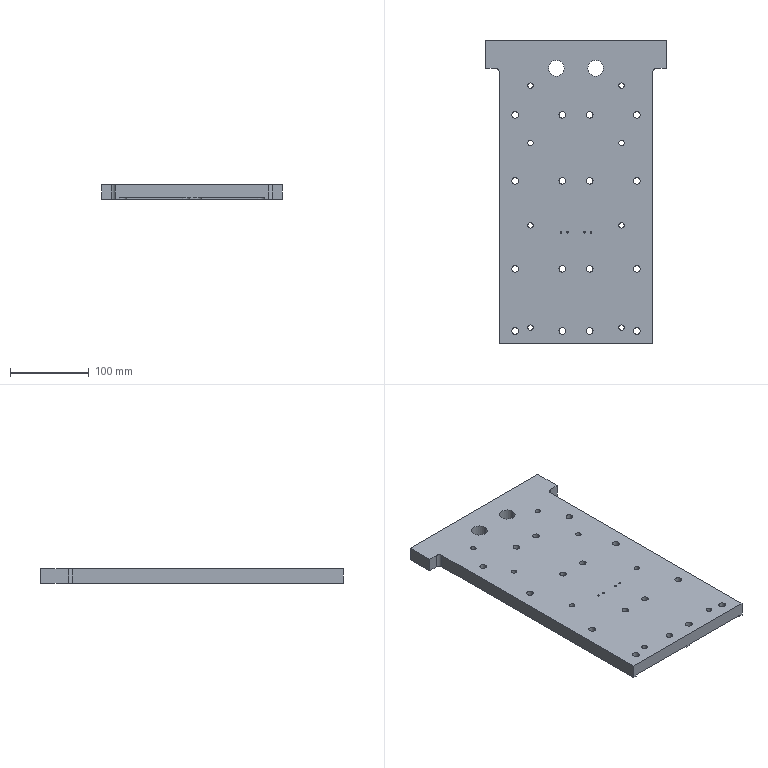NC program | NX | posted with a generic post | part box 230 x 385 x 18 mm
Lines 84 to 1017 of 3056:
(ZLEVEL_PROFILE , TOOL : D10)
N154 T15 M6
N156 G54
N158 G17 G0 G90 X-67.117 Y102.6 S9500 M3
N160 G43 Z30. H15
N162 Z1.5
N164 G94 G1 X-20.05 Z-0.967 F1000.
N166 X152.4 F3000.
N168 Y115.
N170 G2 X157.5 Y120.1 R5.1
N172 G1 X192.5
N174 G2 X197.6 Y115. R5.1
N176 G1 Y-115.
N178 G2 X192.5 Y-120.1 R5.1
N180 G1 X157.5
N182 G2 X152.4 Y-115. R5.1
N184 G1 Y-102.6
N186 X-192.5
N188 G2 X-197.6 Y-97.5 R5.1
N190 G1 Y97.5
N192 G2 X-192.5 Y102.6 R5.1
N194 G1 X-20.05
N196 X152.4 Z-1.099
N198 Y115. Z-1.109
N200 X152.425 Y115.5
N202 X152.498 Y115.995 Z-1.11
N204 X152.62 Y116.48
N206 X152.788 Y116.952
N208 X153.002 Y117.404 Z-1.111
N210 X153.26 Y117.833
N212 X153.558 Y118.235
N214 X153.894 Y118.606 Z-1.112
N216 X154.265 Y118.942
N218 X154.667 Y119.24 Z-1.113
N220 X155.096 Y119.498
N222 X155.548 Y119.712
N224 X156.02 Y119.88 Z-1.114
N226 X156.505 Y120.002
N228 X157. Y120.075 Z-1.115
N230 X157.5 Y120.1
N232 X192.5 Z-1.142
N234 X193. Y120.075
N236 X193.495 Y120.002 Z-1.143
N238 X193.98 Y119.88
N240 X194.452 Y119.712
N242 X194.904 Y119.498 Z-1.144
N244 X195.333 Y119.24
N246 X195.735 Y118.942
N248 X196.106 Y118.606 Z-1.145
N250 X196.442 Y118.235
N252 X196.74 Y117.833 Z-1.146
N254 X196.998 Y117.404
N256 X197.212 Y116.952
N258 X197.38 Y116.48 Z-1.147
N260 X197.502 Y115.995
N262 X197.575 Y115.5 Z-1.148
N264 X197.6 Y115.
N266 Y-115. Z-1.325
N268 X197.575 Y-115.5
N270 X197.502 Y-115.995 Z-1.326
N272 X197.38 Y-116.48
N274 X197.212 Y-116.952
N276 X196.998 Y-117.404 Z-1.327
N278 X196.74 Y-117.833
N280 X196.442 Y-118.235
N282 X196.106 Y-118.606 Z-1.328
N284 X195.735 Y-118.942
N286 X195.333 Y-119.24 Z-1.329
N288 X194.904 Y-119.498
N290 X194.452 Y-119.712
N292 X193.98 Y-119.88 Z-1.33
N294 X193.495 Y-120.002
N296 X193. Y-120.075 Z-1.331
N298 X192.5 Y-120.1
N300 X157.5 Z-1.358
N302 X157. Y-120.075
N304 X156.505 Y-120.002 Z-1.359
N306 X156.02 Y-119.88
N308 X155.548 Y-119.712
N310 X155.096 Y-119.498 Z-1.36
N312 X154.667 Y-119.24
N314 X154.265 Y-118.942
N316 X153.894 Y-118.606 Z-1.361
N318 X153.558 Y-118.235
N320 X153.26 Y-117.833 Z-1.362
N322 X153.002 Y-117.404
N324 X152.788 Y-116.952
N326 X152.62 Y-116.48 Z-1.363
N328 X152.498 Y-115.995
N330 X152.425 Y-115.5 Z-1.364
N332 X152.4 Y-115.
N334 Y-102.6 Z-1.373
N336 X-192.5 Z-1.639
N338 X-193. Y-102.575
N340 X-193.495 Y-102.502
N342 X-193.98 Y-102.38 Z-1.64
N344 X-194.452 Y-102.212
N346 X-194.904 Y-101.998 Z-1.641
N348 X-195.333 Y-101.74
N350 X-195.735 Y-101.442
N352 X-196.106 Y-101.106 Z-1.642
N354 X-196.442 Y-100.735
N356 X-196.74 Y-100.333
N358 X-196.998 Y-99.904 Z-1.643
N360 X-197.212 Y-99.452
N362 X-197.38 Y-98.98 Z-1.644
N364 X-197.502 Y-98.495
N366 X-197.575 Y-98.
N368 X-197.6 Y-97.5 Z-1.645
N370 Y97.5 Z-1.795
N372 X-197.575 Y98.
N374 X-197.502 Y98.495
N376 X-197.38 Y98.98 Z-1.796
N378 X-197.212 Y99.452
N380 X-196.998 Y99.904 Z-1.797
N382 X-196.74 Y100.333
N384 X-196.442 Y100.735
N386 X-196.106 Y101.106 Z-1.798
N388 X-195.735 Y101.442
N390 X-195.333 Y101.74
N392 X-194.904 Y101.998 Z-1.799
N394 X-194.452 Y102.212
N396 X-193.98 Y102.38 Z-1.8
N398 X-193.495 Y102.502
N400 X-193. Y102.575
N402 X-192.5 Y102.6 Z-1.801
N404 X-20.05 Z-1.933
N406 X152.4 Z-2.066
N408 Y115. Z-2.075
N410 X152.425 Y115.5 Z-2.076
N412 X152.498 Y115.995
N414 X152.62 Y116.48 Z-2.077
N416 X152.788 Y116.952
N418 X153.002 Y117.404
N420 X153.26 Y117.833 Z-2.078
N422 X153.558 Y118.235
N424 X153.894 Y118.606
N426 X154.265 Y118.942 Z-2.079
N428 X154.667 Y119.24
N430 X155.096 Y119.498 Z-2.08
N432 X155.548 Y119.712
N434 X156.02 Y119.88
N436 X156.505 Y120.002 Z-2.081
N438 X157. Y120.075
N440 X157.5 Y120.1 Z-2.082
N442 X192.5 Z-2.108
N444 X193. Y120.075 Z-2.109
N446 X193.495 Y120.002
N448 X193.98 Y119.88 Z-2.11
N450 X194.452 Y119.712
N452 X194.904 Y119.498
N454 X195.333 Y119.24 Z-2.111
N456 X195.735 Y118.942
N458 X196.106 Y118.606 Z-2.112
N460 X196.442 Y118.235
N462 X196.74 Y117.833
N464 X196.998 Y117.404 Z-2.113
N466 X197.212 Y116.952
N468 X197.38 Y116.48
N470 X197.502 Y115.995 Z-2.114
N472 X197.575 Y115.5
N474 X197.6 Y115. Z-2.115
N476 Y-115. Z-2.291
N478 X197.575 Y-115.5 Z-2.292
N480 X197.502 Y-115.995
N482 X197.38 Y-116.48 Z-2.293
N484 X197.212 Y-116.952
N486 X196.998 Y-117.404
N488 X196.74 Y-117.833 Z-2.294
N490 X196.442 Y-118.235
N492 X196.106 Y-118.606
N494 X195.735 Y-118.942 Z-2.295
N496 X195.333 Y-119.24
N498 X194.904 Y-119.498 Z-2.296
N500 X194.452 Y-119.712
N502 X193.98 Y-119.88
N504 X193.495 Y-120.002 Z-2.297
N506 X193. Y-120.075
N508 X192.5 Y-120.1 Z-2.298
N510 X157.5 Z-2.324
N512 X157. Y-120.075 Z-2.325
N514 X156.505 Y-120.002
N516 X156.02 Y-119.88 Z-2.326
N518 X155.548 Y-119.712
N520 X155.096 Y-119.498
N522 X154.667 Y-119.24 Z-2.327
N524 X154.265 Y-118.942
N526 X153.894 Y-118.606 Z-2.328
N528 X153.558 Y-118.235
N530 X153.26 Y-117.833
N532 X153.002 Y-117.404 Z-2.329
N534 X152.788 Y-116.952
N536 X152.62 Y-116.48
N538 X152.498 Y-115.995 Z-2.33
N540 X152.425 Y-115.5
N542 X152.4 Y-115. Z-2.331
N544 Y-102.6 Z-2.34
N546 X-192.5 Z-2.605
N548 X-193. Y-102.575 Z-2.606
N550 X-193.495 Y-102.502
N552 X-193.98 Y-102.38
N554 X-194.452 Y-102.212 Z-2.607
N556 X-194.904 Y-101.998
N558 X-195.333 Y-101.74 Z-2.608
N560 X-195.735 Y-101.442
N562 X-196.106 Y-101.106
N564 X-196.442 Y-100.735 Z-2.609
N566 X-196.74 Y-100.333
N568 X-196.998 Y-99.904
N570 X-197.212 Y-99.452 Z-2.61
N572 X-197.38 Y-98.98
N574 X-197.502 Y-98.495 Z-2.611
N576 X-197.575 Y-98.
N578 X-197.6 Y-97.5
N580 Y97.5 Z-2.761
N582 X-197.575 Y98. Z-2.762
N584 X-197.502 Y98.495
N586 X-197.38 Y98.98
N588 X-197.212 Y99.452 Z-2.763
N590 X-196.998 Y99.904
N592 X-196.74 Y100.333 Z-2.764
N594 X-196.442 Y100.735
N596 X-196.106 Y101.106
N598 X-195.735 Y101.442 Z-2.765
N600 X-195.333 Y101.74
N602 X-194.904 Y101.998 Z-2.766
N604 X-194.452 Y102.212
N606 X-193.98 Y102.38
N608 X-193.495 Y102.502 Z-2.767
N610 X-193. Y102.575
N612 X-192.5 Y102.6
N614 X-20.05 Z-2.9
N616 X152.4 Z-3.033
N618 Y115. Z-3.042
N620 X152.425 Y115.5
N622 X152.498 Y115.995 Z-3.043
N624 X152.62 Y116.48
N626 X152.788 Y116.952 Z-3.044
N628 X153.002 Y117.404
N630 X153.26 Y117.833
N632 X153.558 Y118.235 Z-3.045
N634 X153.894 Y118.606
N636 X154.265 Y118.942 Z-3.046
N638 X154.667 Y119.24
N640 X155.096 Y119.498
N642 X155.548 Y119.712 Z-3.047
N644 X156.02 Y119.88
N646 X156.505 Y120.002
N648 X157. Y120.075 Z-3.048
N650 X157.5 Y120.1
N652 X192.5 Z-3.075
N654 X193. Y120.075 Z-3.076
N656 X193.495 Y120.002
N658 X193.98 Y119.88
N660 X194.452 Y119.712 Z-3.077
N662 X194.904 Y119.498
N664 X195.333 Y119.24
N666 X195.735 Y118.942 Z-3.078
N668 X196.106 Y118.606
N670 X196.442 Y118.235 Z-3.079
N672 X196.74 Y117.833
N674 X196.998 Y117.404
N676 X197.212 Y116.952 Z-3.08
N678 X197.38 Y116.48
N680 X197.502 Y115.995 Z-3.081
N682 X197.575 Y115.5
N684 X197.6 Y115.
N686 Y-115. Z-3.258
N688 X197.575 Y-115.5
N690 X197.502 Y-115.995 Z-3.259
N692 X197.38 Y-116.48
N694 X197.212 Y-116.952 Z-3.26
N696 X196.998 Y-117.404
N698 X196.74 Y-117.833
N700 X196.442 Y-118.235 Z-3.261
N702 X196.106 Y-118.606
N704 X195.735 Y-118.942 Z-3.262
N706 X195.333 Y-119.24
N708 X194.904 Y-119.498
N710 X194.452 Y-119.712 Z-3.263
N712 X193.98 Y-119.88
N714 X193.495 Y-120.002
N716 X193. Y-120.075 Z-3.264
N718 X192.5 Y-120.1
N720 X157.5 Z-3.291
N722 X157. Y-120.075 Z-3.292
N724 X156.505 Y-120.002
N726 X156.02 Y-119.88
N728 X155.548 Y-119.712 Z-3.293
N730 X155.096 Y-119.498
N732 X154.667 Y-119.24
N734 X154.265 Y-118.942 Z-3.294
N736 X153.894 Y-118.606
N738 X153.558 Y-118.235 Z-3.295
N740 X153.26 Y-117.833
N742 X153.002 Y-117.404
N744 X152.788 Y-116.952 Z-3.296
N746 X152.62 Y-116.48
N748 X152.498 Y-115.995 Z-3.297
N750 X152.425 Y-115.5
N752 X152.4 Y-115.
N754 Y-102.6 Z-3.307
N756 X-192.5 Z-3.572
N758 X-193. Y-102.575
N760 X-193.495 Y-102.502 Z-3.573
N762 X-193.98 Y-102.38
N764 X-194.452 Y-102.212
N766 X-194.904 Y-101.998 Z-3.574
N768 X-195.333 Y-101.74
N770 X-195.735 Y-101.442 Z-3.575
N772 X-196.106 Y-101.106
N774 X-196.442 Y-100.735
N776 X-196.74 Y-100.333 Z-3.576
N778 X-196.998 Y-99.904
N780 X-197.212 Y-99.452 Z-3.577
N782 X-197.38 Y-98.98
N784 X-197.502 Y-98.495
N786 X-197.575 Y-98. Z-3.578
N788 X-197.6 Y-97.5
N790 Y97.5 Z-3.728
N792 X-197.575 Y98.
N794 X-197.502 Y98.495 Z-3.729
N796 X-197.38 Y98.98
N798 X-197.212 Y99.452 Z-3.73
N800 X-196.998 Y99.904
N802 X-196.74 Y100.333
N804 X-196.442 Y100.735 Z-3.731
N806 X-196.106 Y101.106
N808 X-195.735 Y101.442
N810 X-195.333 Y101.74 Z-3.732
N812 X-194.904 Y101.998
N814 X-194.452 Y102.212 Z-3.733
N816 X-193.98 Y102.38
N818 X-193.495 Y102.502
N820 X-193. Y102.575 Z-3.734
N822 X-192.5 Y102.6
N824 X-20.05 Z-3.867
N826 X152.4 Z-3.999
N828 Y115. Z-4.009
N830 X152.425 Y115.5
N832 X152.498 Y115.995 Z-4.01
N834 X152.62 Y116.48
N836 X152.788 Y116.952
N838 X153.002 Y117.404 Z-4.011
N840 X153.26 Y117.833
N842 X153.558 Y118.235
N844 X153.894 Y118.606 Z-4.012
N846 X154.265 Y118.942
N848 X154.667 Y119.24 Z-4.013
N850 X155.096 Y119.498
N852 X155.548 Y119.712
N854 X156.02 Y119.88 Z-4.014
N856 X156.505 Y120.002
N858 X157. Y120.075 Z-4.015
N860 X157.5 Y120.1
N862 X192.5 Z-4.042
N864 X193. Y120.075
N866 X193.495 Y120.002 Z-4.043
N868 X193.98 Y119.88
N870 X194.452 Y119.712
N872 X194.904 Y119.498 Z-4.044
N874 X195.333 Y119.24
N876 X195.735 Y118.942
N878 X196.106 Y118.606 Z-4.045
N880 X196.442 Y118.235
N882 X196.74 Y117.833 Z-4.046
N884 X196.998 Y117.404
N886 X197.212 Y116.952
N888 X197.38 Y116.48 Z-4.047
N890 X197.502 Y115.995
N892 X197.575 Y115.5 Z-4.048
N894 X197.6 Y115.
N896 Y-115. Z-4.225
N898 X197.575 Y-115.5
N900 X197.502 Y-115.995 Z-4.226
N902 X197.38 Y-116.48
N904 X197.212 Y-116.952
N906 X196.998 Y-117.404 Z-4.227
N908 X196.74 Y-117.833
N910 X196.442 Y-118.235
N912 X196.106 Y-118.606 Z-4.228
N914 X195.735 Y-118.942
N916 X195.333 Y-119.24 Z-4.229
N918 X194.904 Y-119.498
N920 X194.452 Y-119.712
N922 X193.98 Y-119.88 Z-4.23
N924 X193.495 Y-120.002
N926 X193. Y-120.075 Z-4.231
N928 X192.5 Y-120.1
N930 X157.5 Z-4.258
N932 X157. Y-120.075
N934 X156.505 Y-120.002 Z-4.259
N936 X156.02 Y-119.88
N938 X155.548 Y-119.712
N940 X155.096 Y-119.498 Z-4.26
N942 X154.667 Y-119.24
N944 X154.265 Y-118.942
N946 X153.894 Y-118.606 Z-4.261
N948 X153.558 Y-118.235
N950 X153.26 Y-117.833 Z-4.262
N952 X153.002 Y-117.404
N954 X152.788 Y-116.952
N956 X152.62 Y-116.48 Z-4.263
N958 X152.498 Y-115.995
N960 X152.425 Y-115.5 Z-4.264
N962 X152.4 Y-115.
N964 Y-102.6 Z-4.273
N966 X-192.5 Z-4.539
N968 X-193. Y-102.575
N970 X-193.495 Y-102.502
N972 X-193.98 Y-102.38 Z-4.54
N974 X-194.452 Y-102.212
N976 X-194.904 Y-101.998 Z-4.541
N978 X-195.333 Y-101.74
N980 X-195.735 Y-101.442
N982 X-196.106 Y-101.106 Z-4.542
N984 X-196.442 Y-100.735
N986 X-196.74 Y-100.333
N988 X-196.998 Y-99.904 Z-4.543
N990 X-197.212 Y-99.452
N992 X-197.38 Y-98.98 Z-4.544
N994 X-197.502 Y-98.495
N996 X-197.575 Y-98.
N998 X-197.6 Y-97.5 Z-4.545
N1000 Y97.5 Z-4.695
N1002 X-197.575 Y98.
N1004 X-197.502 Y98.495
N1006 X-197.38 Y98.98 Z-4.696
N1008 X-197.212 Y99.452
N1010 X-196.998 Y99.904 Z-4.697
N1012 X-196.74 Y100.333
N1014 X-196.442 Y100.735
N1016 X-196.106 Y101.106 Z-4.698
N1018 X-195.735 Y101.442
N1020 X-195.333 Y101.74
N1022 X-194.904 Y101.998 Z-4.699
N1024 X-194.452 Y102.212
N1026 X-193.98 Y102.38 Z-4.7
N1028 X-193.495 Y102.502
N1030 X-193. Y102.575
N1032 X-192.5 Y102.6 Z-4.701
N1034 X-20.05 Z-4.833
N1036 X152.4 Z-4.966
N1038 Y115. Z-4.975
N1040 X152.425 Y115.5 Z-4.976
N1042 X152.498 Y115.995
N1044 X152.62 Y116.48 Z-4.977
N1046 X152.788 Y116.952
N1048 X153.002 Y117.404
N1050 X153.26 Y117.833 Z-4.978
N1052 X153.558 Y118.235
N1054 X153.894 Y118.606
N1056 X154.265 Y118.942 Z-4.979
N1058 X154.667 Y119.24
N1060 X155.096 Y119.498 Z-4.98
N1062 X155.548 Y119.712
N1064 X156.02 Y119.88
N1066 X156.505 Y120.002 Z-4.981
N1068 X157. Y120.075
N1070 X157.5 Y120.1 Z-4.982
N1072 X192.5 Z-5.008
N1074 X193. Y120.075 Z-5.009
N1076 X193.495 Y120.002
N1078 X193.98 Y119.88 Z-5.01
N1080 X194.452 Y119.712
N1082 X194.904 Y119.498
N1084 X195.333 Y119.24 Z-5.011
N1086 X195.735 Y118.942
N1088 X196.106 Y118.606 Z-5.012
N1090 X196.442 Y118.235
N1092 X196.74 Y117.833
N1094 X196.998 Y117.404 Z-5.013
N1096 X197.212 Y116.952
N1098 X197.38 Y116.48
N1100 X197.502 Y115.995 Z-5.014
N1102 X197.575 Y115.5
N1104 X197.6 Y115. Z-5.015
N1106 Y-115. Z-5.191
N1108 X197.575 Y-115.5 Z-5.192
N1110 X197.502 Y-115.995
N1112 X197.38 Y-116.48 Z-5.193
N1114 X197.212 Y-116.952
N1116 X196.998 Y-117.404
N1118 X196.74 Y-117.833 Z-5.194
N1120 X196.442 Y-118.235
N1122 X196.106 Y-118.606
N1124 X195.735 Y-118.942 Z-5.195
N1126 X195.333 Y-119.24
N1128 X194.904 Y-119.498 Z-5.196
N1130 X194.452 Y-119.712
N1132 X193.98 Y-119.88
N1134 X193.495 Y-120.002 Z-5.197
N1136 X193. Y-120.075
N1138 X192.5 Y-120.1 Z-5.198
N1140 X157.5 Z-5.224
N1142 X157. Y-120.075 Z-5.225
N1144 X156.505 Y-120.002
N1146 X156.02 Y-119.88 Z-5.226
N1148 X155.548 Y-119.712
N1150 X155.096 Y-119.498
N1152 X154.667 Y-119.24 Z-5.227
N1154 X154.265 Y-118.942
N1156 X153.894 Y-118.606 Z-5.228
N1158 X153.558 Y-118.235
N1160 X153.26 Y-117.833
N1162 X153.002 Y-117.404 Z-5.229
N1164 X152.788 Y-116.952
N1166 X152.62 Y-116.48
N1168 X152.498 Y-115.995 Z-5.23
N1170 X152.425 Y-115.5
N1172 X152.4 Y-115. Z-5.231
N1174 Y-102.6 Z-5.24
N1176 X-192.5 Z-5.505
N1178 X-193. Y-102.575 Z-5.506
N1180 X-193.495 Y-102.502
N1182 X-193.98 Y-102.38
N1184 X-194.452 Y-102.212 Z-5.507
N1186 X-194.904 Y-101.998
N1188 X-195.333 Y-101.74 Z-5.508
N1190 X-195.735 Y-101.442
N1192 X-196.106 Y-101.106
N1194 X-196.442 Y-100.735 Z-5.509
N1196 X-196.74 Y-100.333
N1198 X-196.998 Y-99.904
N1200 X-197.212 Y-99.452 Z-5.51
N1202 X-197.38 Y-98.98
N1204 X-197.502 Y-98.495 Z-5.511
N1206 X-197.575 Y-98.
N1208 X-197.6 Y-97.5
N1210 Y97.5 Z-5.661
N1212 X-197.575 Y98. Z-5.662
N1214 X-197.502 Y98.495
N1216 X-197.38 Y98.98
N1218 X-197.212 Y99.452 Z-5.663
N1220 X-196.998 Y99.904
N1222 X-196.74 Y100.333 Z-5.664
N1224 X-196.442 Y100.735
N1226 X-196.106 Y101.106
N1228 X-195.735 Y101.442 Z-5.665
N1230 X-195.333 Y101.74
N1232 X-194.904 Y101.998 Z-5.666
N1234 X-194.452 Y102.212
N1236 X-193.98 Y102.38
N1238 X-193.495 Y102.502 Z-5.667
N1240 X-193. Y102.575
N1242 X-192.5 Y102.6
N1244 X-20.05 Z-5.8
N1246 X152.4 Z-5.933
N1248 Y115. Z-5.942
N1250 X152.425 Y115.5
N1252 X152.498 Y115.995 Z-5.943
N1254 X152.62 Y116.48
N1256 X152.788 Y116.952 Z-5.944
N1258 X153.002 Y117.404
N1260 X153.26 Y117.833
N1262 X153.558 Y118.235 Z-5.945
N1264 X153.894 Y118.606
N1266 X154.265 Y118.942 Z-5.946
N1268 X154.667 Y119.24
N1270 X155.096 Y119.498
N1272 X155.548 Y119.712 Z-5.947
N1274 X156.02 Y119.88
N1276 X156.505 Y120.002
N1278 X157. Y120.075 Z-5.948
N1280 X157.5 Y120.1
N1282 X192.5 Z-5.975
N1284 X193. Y120.075 Z-5.976
N1286 X193.495 Y120.002
N1288 X193.98 Y119.88
N1290 X194.452 Y119.712 Z-5.977
N1292 X194.904 Y119.498
N1294 X195.333 Y119.24
N1296 X195.735 Y118.942 Z-5.978
N1298 X196.106 Y118.606
N1300 X196.442 Y118.235 Z-5.979
N1302 X196.74 Y117.833
N1304 X196.998 Y117.404
N1306 X197.212 Y116.952 Z-5.98
N1308 X197.38 Y116.48
N1310 X197.502 Y115.995 Z-5.981
N1312 X197.575 Y115.5
N1314 X197.6 Y115.
N1316 Y-115. Z-6.158
N1318 X197.575 Y-115.5
N1320 X197.502 Y-115.995 Z-6.159
N1322 X197.38 Y-116.48
N1324 X197.212 Y-116.952 Z-6.16
N1326 X196.998 Y-117.404
N1328 X196.74 Y-117.833
N1330 X196.442 Y-118.235 Z-6.161
N1332 X196.106 Y-118.606
N1334 X195.735 Y-118.942 Z-6.162
N1336 X195.333 Y-119.24
N1338 X194.904 Y-119.498
N1340 X194.452 Y-119.712 Z-6.163
N1342 X193.98 Y-119.88
N1344 X193.495 Y-120.002
N1346 X193. Y-120.075 Z-6.164
N1348 X192.5 Y-120.1
N1350 X157.5 Z-6.191
N1352 X157. Y-120.075 Z-6.192
N1354 X156.505 Y-120.002
N1356 X156.02 Y-119.88
N1358 X155.548 Y-119.712 Z-6.193
N1360 X155.096 Y-119.498
N1362 X154.667 Y-119.24
N1364 X154.265 Y-118.942 Z-6.194
N1366 X153.894 Y-118.606
N1368 X153.558 Y-118.235 Z-6.195
N1370 X153.26 Y-117.833
N1372 X153.002 Y-117.404
N1374 X152.788 Y-116.952 Z-6.196
N1376 X152.62 Y-116.48
N1378 X152.498 Y-115.995 Z-6.197
N1380 X152.425 Y-115.5
N1382 X152.4 Y-115.
N1384 Y-102.6 Z-6.207
N1386 X-192.5 Z-6.472
N1388 X-193. Y-102.575
N1390 X-193.495 Y-102.502 Z-6.473
N1392 X-193.98 Y-102.38
N1394 X-194.452 Y-102.212
N1396 X-194.904 Y-101.998 Z-6.474
N1398 X-195.333 Y-101.74
N1400 X-195.735 Y-101.442 Z-6.475
N1402 X-196.106 Y-101.106
N1404 X-196.442 Y-100.735
N1406 X-196.74 Y-100.333 Z-6.476
N1408 X-196.998 Y-99.904
N1410 X-197.212 Y-99.452 Z-6.477
N1412 X-197.38 Y-98.98
N1414 X-197.502 Y-98.495
N1416 X-197.575 Y-98. Z-6.478
N1418 X-197.6 Y-97.5
N1420 Y97.5 Z-6.628
N1422 X-197.575 Y98.
N1424 X-197.502 Y98.495 Z-6.629
N1426 X-197.38 Y98.98
N1428 X-197.212 Y99.452 Z-6.63
N1430 X-196.998 Y99.904
N1432 X-196.74 Y100.333
N1434 X-196.442 Y100.735 Z-6.631
N1436 X-196.106 Y101.106
N1438 X-195.735 Y101.442
N1440 X-195.333 Y101.74 Z-6.632
N1442 X-194.904 Y101.998
N1444 X-194.452 Y102.212 Z-6.633
N1446 X-193.98 Y102.38
N1448 X-193.495 Y102.502
N1450 X-193. Y102.575 Z-6.634
N1452 X-192.5 Y102.6
N1454 X-20.05 Z-6.767
N1456 X152.4 Z-6.899
N1458 Y115. Z-6.909
N1460 X152.425 Y115.5
N1462 X152.498 Y115.995 Z-6.91
N1464 X152.62 Y116.48
N1466 X152.788 Y116.952
N1468 X153.002 Y117.404 Z-6.911
N1470 X153.26 Y117.833
N1472 X153.558 Y118.235
N1474 X153.894 Y118.606 Z-6.912
N1476 X154.265 Y118.942
N1478 X154.667 Y119.24 Z-6.913
N1480 X155.096 Y119.498
N1482 X155.548 Y119.712
N1484 X156.02 Y119.88 Z-6.914
N1486 X156.505 Y120.002
N1488 X157. Y120.075 Z-6.915
N1490 X157.5 Y120.1
N1492 X192.5 Z-6.942
N1494 X193. Y120.075
N1496 X193.495 Y120.002 Z-6.943
N1498 X193.98 Y119.88
N1500 X194.452 Y119.712
N1502 X194.904 Y119.498 Z-6.944
N1504 X195.333 Y119.24
N1506 X195.735 Y118.942
N1508 X196.106 Y118.606 Z-6.945
N1510 X196.442 Y118.235
N1512 X196.74 Y117.833 Z-6.946
N1514 X196.998 Y117.404
N1516 X197.212 Y116.952
N1518 X197.38 Y116.48 Z-6.947
N1520 X197.502 Y115.995
N1522 X197.575 Y115.5 Z-6.948
N1524 X197.6 Y115.
N1526 Y-115. Z-7.125
N1528 X197.575 Y-115.5
N1530 X197.502 Y-115.995 Z-7.126
N1532 X197.38 Y-116.48
N1534 X197.212 Y-116.952
N1536 X196.998 Y-117.404 Z-7.127
N1538 X196.74 Y-117.833
N1540 X196.442 Y-118.235
N1542 X196.106 Y-118.606 Z-7.128
N1544 X195.735 Y-118.942
N1546 X195.333 Y-119.24 Z-7.129
N1548 X194.904 Y-119.498
N1550 X194.452 Y-119.712
N1552 X193.98 Y-119.88 Z-7.13
N1554 X193.495 Y-120.002
N1556 X193. Y-120.075 Z-7.131
N1558 X192.5 Y-120.1
N1560 X157.5 Z-7.158
N1562 X157. Y-120.075
N1564 X156.505 Y-120.002 Z-7.159
N1566 X156.02 Y-119.88
N1568 X155.548 Y-119.712
N1570 X155.096 Y-119.498 Z-7.16
N1572 X154.667 Y-119.24
N1574 X154.265 Y-118.942
N1576 X153.894 Y-118.606 Z-7.161
N1578 X153.558 Y-118.235
N1580 X153.26 Y-117.833 Z-7.162
N1582 X153.002 Y-117.404
N1584 X152.788 Y-116.952
N1586 X152.62 Y-116.48 Z-7.163
N1588 X152.498 Y-115.995
N1590 X152.425 Y-115.5 Z-7.164
N1592 X152.4 Y-115.
N1594 Y-102.6 Z-7.173
N1596 X-192.5 Z-7.439
N1598 X-193. Y-102.575
N1600 X-193.495 Y-102.502
N1602 X-193.98 Y-102.38 Z-7.44
N1604 X-194.452 Y-102.212
N1606 X-194.904 Y-101.998 Z-7.441
N1608 X-195.333 Y-101.74
N1610 X-195.735 Y-101.442
N1612 X-196.106 Y-101.106 Z-7.442
N1614 X-196.442 Y-100.735
N1616 X-196.74 Y-100.333
N1618 X-196.998 Y-99.904 Z-7.443
N1620 X-197.212 Y-99.452
N1622 X-197.38 Y-98.98 Z-7.444
N1624 X-197.502 Y-98.495
N1626 X-197.575 Y-98.
N1628 X-197.6 Y-97.5 Z-7.445
N1630 Y97.5 Z-7.595
N1632 X-197.575 Y98.
N1634 X-197.502 Y98.495
N1636 X-197.38 Y98.98 Z-7.596
N1638 X-197.212 Y99.452
N1640 X-196.998 Y99.904 Z-7.597
N1642 X-196.74 Y100.333
N1644 X-196.442 Y100.735
N1646 X-196.106 Y101.106 Z-7.598
N1648 X-195.735 Y101.442
N1650 X-195.333 Y101.74
N1652 X-194.904 Y101.998 Z-7.599
N1654 X-194.452 Y102.212
N1656 X-193.98 Y102.38 Z-7.6
N1658 X-193.495 Y102.502
N1660 X-193. Y102.575
N1662 X-192.5 Y102.6 Z-7.601
N1664 X-20.05 Z-7.733
N1666 X152.4 Z-7.866
N1668 Y115. Z-7.875
N1670 X152.425 Y115.5 Z-7.876
N1672 X152.498 Y115.995
N1674 X152.62 Y116.48 Z-7.877
N1676 X152.788 Y116.952
N1678 X153.002 Y117.404
N1680 X153.26 Y117.833 Z-7.878
N1682 X153.558 Y118.235
N1684 X153.894 Y118.606
N1686 X154.265 Y118.942 Z-7.879
N1688 X154.667 Y119.24
N1690 X155.096 Y119.498 Z-7.88
N1692 X155.548 Y119.712
N1694 X156.02 Y119.88
N1696 X156.505 Y120.002 Z-7.881
N1698 X157. Y120.075
N1700 X157.5 Y120.1 Z-7.882
N1702 X192.5 Z-7.908
N1704 X193. Y120.075 Z-7.909
N1706 X193.495 Y120.002
N1708 X193.98 Y119.88 Z-7.91
N1710 X194.452 Y119.712
N1712 X194.904 Y119.498
N1714 X195.333 Y119.24 Z-7.911
N1716 X195.735 Y118.942
N1718 X196.106 Y118.606 Z-7.912
N1720 X196.442 Y118.235
N1722 X196.74 Y117.833
N1724 X196.998 Y117.404 Z-7.913
N1726 X197.212 Y116.952
N1728 X197.38 Y116.48
N1730 X197.502 Y115.995 Z-7.914
N1732 X197.575 Y115.5
N1734 X197.6 Y115. Z-7.915
N1736 Y-115. Z-8.091
N1738 X197.575 Y-115.5 Z-8.092
N1740 X197.502 Y-115.995
N1742 X197.38 Y-116.48 Z-8.093
N1744 X197.212 Y-116.952
N1746 X196.998 Y-117.404
N1748 X196.74 Y-117.833 Z-8.094
N1750 X196.442 Y-118.235
N1752 X196.106 Y-118.606
N1754 X195.735 Y-118.942 Z-8.095
N1756 X195.333 Y-119.24
N1758 X194.904 Y-119.498 Z-8.096
N1760 X194.452 Y-119.712
N1762 X193.98 Y-119.88
N1764 X193.495 Y-120.002 Z-8.097
N1766 X193. Y-120.075
N1768 X192.5 Y-120.1 Z-8.098
N1770 X157.5 Z-8.124
N1772 X157. Y-120.075 Z-8.125
N1774 X156.505 Y-120.002
N1776 X156.02 Y-119.88 Z-8.126
N1778 X155.548 Y-119.712
N1780 X155.096 Y-119.498
N1782 X154.667 Y-119.24 Z-8.127
N1784 X154.265 Y-118.942
N1786 X153.894 Y-118.606 Z-8.128
N1788 X153.558 Y-118.235
N1790 X153.26 Y-117.833
N1792 X153.002 Y-117.404 Z-8.129
N1794 X152.788 Y-116.952
N1796 X152.62 Y-116.48
N1798 X152.498 Y-115.995 Z-8.13
N1800 X152.425 Y-115.5
N1802 X152.4 Y-115. Z-8.131
N1804 Y-102.6 Z-8.14
N1806 X-192.5 Z-8.405
N1808 X-193. Y-102.575 Z-8.406
N1810 X-193.495 Y-102.502
N1812 X-193.98 Y-102.38
N1814 X-194.452 Y-102.212 Z-8.407
N1816 X-194.904 Y-101.998
N1818 X-195.333 Y-101.74 Z-8.408
N1820 X-195.735 Y-101.442
N1822 X-196.106 Y-101.106
N1824 X-196.442 Y-100.735 Z-8.409
N1826 X-196.74 Y-100.333
N1828 X-196.998 Y-99.904
N1830 X-197.212 Y-99.452 Z-8.41
N1832 X-197.38 Y-98.98
N1834 X-197.502 Y-98.495 Z-8.411
N1836 X-197.575 Y-98.
N1838 X-197.6 Y-97.5
N1840 Y97.5 Z-8.561
N1842 X-197.575 Y98. Z-8.562
N1844 X-197.502 Y98.495
N1846 X-197.38 Y98.98
N1848 X-197.212 Y99.452 Z-8.563
N1850 X-196.998 Y99.904
N1852 X-196.74 Y100.333 Z-8.564
N1854 X-196.442 Y100.735
N1856 X-196.106 Y101.106
N1858 X-195.735 Y101.442 Z-8.565
N1860 X-195.333 Y101.74
N1862 X-194.904 Y101.998 Z-8.566
N1864 X-194.452 Y102.212
N1866 X-193.98 Y102.38
N1868 X-193.495 Y102.502 Z-8.567
N1870 X-193. Y102.575
N1872 X-192.5 Y102.6
N1874 X-20.05 Z-8.7
N1876 X152.4 Z-8.833
N1878 Y115. Z-8.842
N1880 X152.425 Y115.5
N1882 X152.498 Y115.995 Z-8.843
N1884 X152.62 Y116.48
N1886 X152.788 Y116.952 Z-8.844
N1888 X153.002 Y117.404
N1890 X153.26 Y117.833
N1892 X153.558 Y118.235 Z-8.845
N1894 X153.894 Y118.606
N1896 X154.265 Y118.942 Z-8.846
N1898 X154.667 Y119.24
N1900 X155.096 Y119.498
N1902 X155.548 Y119.712 Z-8.847
N1904 X156.02 Y119.88
N1906 X156.505 Y120.002
N1908 X157. Y120.075 Z-8.848
N1910 X157.5 Y120.1
N1912 X192.5 Z-8.875
N1914 X193. Y120.075 Z-8.876
N1916 X193.495 Y120.002
N1918 X193.98 Y119.88
N1920 X194.452 Y119.712 Z-8.877
N1922 X194.904 Y119.498
N1924 X195.333 Y119.24
N1926 X195.735 Y118.942 Z-8.878
N1928 X196.106 Y118.606
N1930 X196.442 Y118.235 Z-8.879
N1932 X196.74 Y117.833
N1934 X196.998 Y117.404
N1936 X197.212 Y116.952 Z-8.88
N1938 X197.38 Y116.48
N1940 X197.502 Y115.995 Z-8.881
N1942 X197.575 Y115.5
N1944 X197.6 Y115.
N1946 Y-115. Z-9.058
N1948 X197.575 Y-115.5
N1950 X197.502 Y-115.995 Z-9.059
N1952 X197.38 Y-116.48
N1954 X197.212 Y-116.952 Z-9.06
N1956 X196.998 Y-117.404
N1958 X196.74 Y-117.833
N1960 X196.442 Y-118.235 Z-9.061
N1962 X196.106 Y-118.606
N1964 X195.735 Y-118.942 Z-9.062
N1966 X195.333 Y-119.24
N1968 X194.904 Y-119.498
N1970 X194.452 Y-119.712 Z-9.063
N1972 X193.98 Y-119.88
N1974 X193.495 Y-120.002
N1976 X193. Y-120.075 Z-9.064
N1978 X192.5 Y-120.1
N1980 X157.5 Z-9.091
N1982 X157. Y-120.075 Z-9.092
N1984 X156.505 Y-120.002
N1986 X156.02 Y-119.88
N1988 X155.548 Y-119.712 Z-9.093
N1990 X155.096 Y-119.498
N1992 X154.667 Y-119.24
N1994 X154.265 Y-118.942 Z-9.094
N1996 X153.894 Y-118.606
N1998 X153.558 Y-118.235 Z-9.095
N2000 X153.26 Y-117.833
N2002 X153.002 Y-117.404
N2004 X152.788 Y-116.952 Z-9.096
N2006 X152.62 Y-116.48
N2008 X152.498 Y-115.995 Z-9.097
N2010 X152.425 Y-115.5
N2012 X152.4 Y-115.
N2014 Y-102.6 Z-9.107